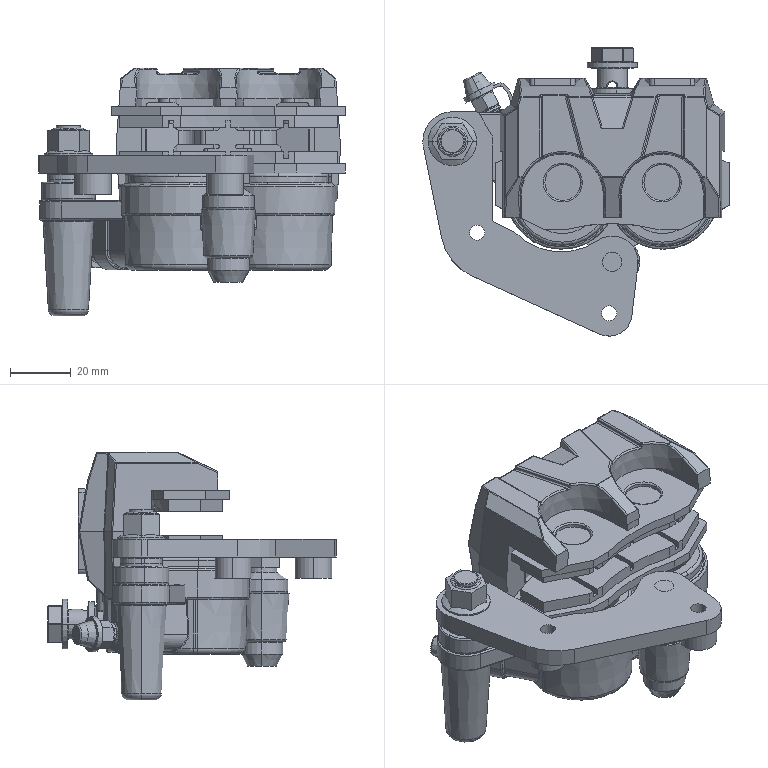Part | SolidWorks | 20 solids | 1154 faces | box 100.95 x 95.04 x 81.512 mm | volume 159113 mm3 | cylinder 505 | plane 380 | torus 88 | cone 78 | spline 68 | sphere 35 | commonest cylinder face diameters 1 x112 8 x38 9.8 x38 4 x27 9.82 x24 2 x19